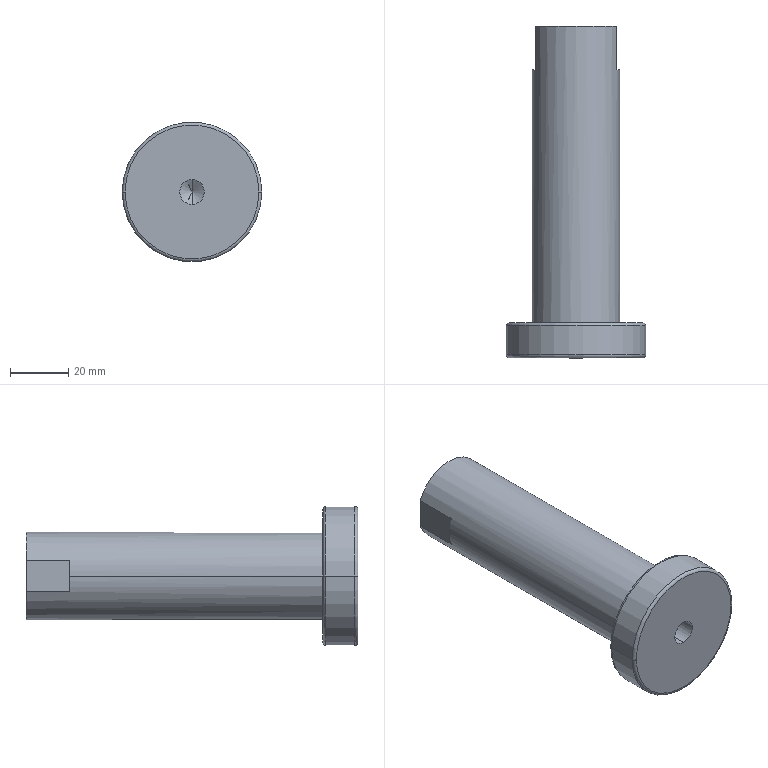Part | SolidWorks | features HoleWzd 2, Fillet 1, ICE 1, Revolution 1 | 1 solid | 23 faces | box 48 x 114 x 48 mm | volume 74222 mm3 | cylinder 8 | plane 7 | cone 4 | torus 4 | commonest cylinder face diameters 8.5 x2 24.5 x2 30 x2 48 x2
STEP:
#1=CARTESIAN_POINT('',(0.,-1.947,4.25));
#2=VERTEX_POINT('',#1);
#3=CARTESIAN_POINT('',(0.,-1.947,-4.25));
#4=VERTEX_POINT('',#3);
#5=CARTESIAN_POINT('',(0.,-1.947,0.));
#6=DIRECTION('',(0.,-1.,0.));
#7=DIRECTION('',(0.,0.,-1.));
#8=AXIS2_PLACEMENT_3D('',#5,#6,#7);
#9=CIRCLE('',#8,4.25);
#10=EDGE_CURVE('',#2,#4,#9,.T.);
#11=ORIENTED_EDGE('',*,*,#10,.F.);
#12=CARTESIAN_POINT('',(0.,-21.947,4.25));
#13=VERTEX_POINT('',#12);
#14=CARTESIAN_POINT('',(0.,-21.947,4.25));
#15=DIRECTION('',(0.,-1.,0.));
#16=VECTOR('',#15,1000.);
#17=LINE('',#14,#16);
#18=EDGE_CURVE('',#2,#13,#17,.T.);
#19=ORIENTED_EDGE('',*,*,#18,.T.);
#20=CARTESIAN_POINT('',(0.,-21.947,-4.25));
#21=VERTEX_POINT('',#20);
#22=CARTESIAN_POINT('',(0.,-21.947,0.));
#23=DIRECTION('',(0.,-1.,0.));
#24=DIRECTION('',(0.,0.,-1.));
#25=AXIS2_PLACEMENT_3D('',#22,#23,#24);
#26=CIRCLE('',#25,4.25);
#27=EDGE_CURVE('',#13,#21,#26,.T.);
#28=ORIENTED_EDGE('',*,*,#27,.T.);
#29=CARTESIAN_POINT('',(0.,-21.947,-4.25));
#30=DIRECTION('',(0.,-1.,0.));
#31=VECTOR('',#30,1000.);
#32=LINE('',#29,#31);
#33=EDGE_CURVE('',#4,#21,#32,.T.);
#34=ORIENTED_EDGE('',*,*,#33,.F.);
#35=EDGE_LOOP('',(#11,#19,#28,#34));
#36=FACE_OUTER_BOUND('',#35,.T.);
#37=CARTESIAN_POINT('',(0.,-21.947,0.));
#38=DIRECTION('',(0.,-1.,0.));
#39=DIRECTION('',(0.,0.,-1.));
#40=AXIS2_PLACEMENT_3D('',#37,#38,#39);
#41=CYLINDRICAL_SURFACE('',#40,4.25);
#42=ADVANCED_FACE('',(#36),#41,.F.);
#43=CARTESIAN_POINT('',(0.,0.6063,0.));
#44=VERTEX_POINT('',#43);
#45=CARTESIAN_POINT('',(0.,-1.947,-4.25));
#46=DIRECTION('',(0.,-0.515,-0.8572));
#47=VECTOR('',#46,1000.);
#48=LINE('',#45,#47);
#49=EDGE_CURVE('',#44,#4,#48,.T.);
#50=ORIENTED_EDGE('',*,*,#49,.F.);
#51=CARTESIAN_POINT('',(0.,-1.947,4.25));
#52=DIRECTION('',(0.,-0.515,0.8572));
#53=VECTOR('',#52,1000.);
#54=LINE('',#51,#53);
#55=EDGE_CURVE('',#44,#2,#54,.T.);
#56=ORIENTED_EDGE('',*,*,#55,.T.);
#57=ORIENTED_EDGE('',*,*,#10,.T.);
#58=EDGE_LOOP('',(#50,#56,#57));
#59=FACE_OUTER_BOUND('',#58,.T.);
#60=CARTESIAN_POINT('',(0.,-1.947,0.));
#61=DIRECTION('',(0.,-1.,0.));
#62=DIRECTION('',(0.,0.,-1.));
#63=AXIS2_PLACEMENT_3D('',#60,#61,#62);
#64=CONICAL_SURFACE('',#63,4.25,1.03);
#65=ADVANCED_FACE('',(#59),#64,.F.);
#66=CARTESIAN_POINT('',(0.,56.053,-12.25));
#67=VERTEX_POINT('',#66);
#68=CARTESIAN_POINT('',(0.,56.053,12.25));
#69=VERTEX_POINT('',#68);
#70=CARTESIAN_POINT('',(0.,56.053,0.));
#71=DIRECTION('',(0.,1.,0.));
#72=DIRECTION('',(0.,0.,1.));
#73=AXIS2_PLACEMENT_3D('',#70,#71,#72);
#74=CIRCLE('',#73,12.25);
#75=EDGE_CURVE('',#67,#69,#74,.T.);
#76=ORIENTED_EDGE('',*,*,#75,.F.);
#77=CARTESIAN_POINT('',(0.,92.053,-12.25));
#78=VERTEX_POINT('',#77);
#79=CARTESIAN_POINT('',(0.,92.053,-12.25));
#80=DIRECTION('',(0.,1.,0.));
#81=VECTOR('',#80,1000.);
#82=LINE('',#79,#81);
#83=EDGE_CURVE('',#67,#78,#82,.T.);
#84=ORIENTED_EDGE('',*,*,#83,.T.);
#85=CARTESIAN_POINT('',(0.,92.053,12.25));
#86=VERTEX_POINT('',#85);
#87=CARTESIAN_POINT('',(0.,92.053,0.));
#88=DIRECTION('',(0.,1.,0.));
#89=DIRECTION('',(0.,0.,1.));
#90=AXIS2_PLACEMENT_3D('',#87,#88,#89);
#91=CIRCLE('',#90,12.25);
#92=EDGE_CURVE('',#78,#86,#91,.T.);
#93=ORIENTED_EDGE('',*,*,#92,.T.);
#94=CARTESIAN_POINT('',(0.,92.053,12.25));
#95=DIRECTION('',(0.,1.,0.));
#96=VECTOR('',#95,1000.);
#97=LINE('',#94,#96);
#98=EDGE_CURVE('',#69,#86,#97,.T.);
#99=ORIENTED_EDGE('',*,*,#98,.F.);
#100=EDGE_LOOP('',(#76,#84,#93,#99));
#101=FACE_OUTER_BOUND('',#100,.T.);
#102=CARTESIAN_POINT('',(0.,92.053,0.));
#103=DIRECTION('',(0.,1.,0.));
#104=DIRECTION('',(0.,0.,1.));
#105=AXIS2_PLACEMENT_3D('',#102,#103,#104);
#106=CYLINDRICAL_SURFACE('',#105,12.25);
#107=ADVANCED_FACE('',(#101),#106,.F.);
#108=CARTESIAN_POINT('',(0.,48.692,0.));
#109=VERTEX_POINT('',#108);
#110=CARTESIAN_POINT('',(0.,56.053,12.25));
#111=DIRECTION('',(0.,0.515,0.8572));
#112=VECTOR('',#111,1000.);
#113=LINE('',#110,#112);
#114=EDGE_CURVE('',#109,#69,#113,.T.);
#115=ORIENTED_EDGE('',*,*,#114,.F.);
#116=CARTESIAN_POINT('',(0.,56.053,-12.25));
#117=DIRECTION('',(0.,0.515,-0.8572));
#118=VECTOR('',#117,1000.);
#119=LINE('',#116,#118);
#120=EDGE_CURVE('',#109,#67,#119,.T.);
#121=ORIENTED_EDGE('',*,*,#120,.T.);
#122=ORIENTED_EDGE('',*,*,#75,.T.);
#123=EDGE_LOOP('',(#115,#121,#122));
#124=FACE_OUTER_BOUND('',#123,.T.);
#125=CARTESIAN_POINT('',(0.,56.053,0.));
#126=DIRECTION('',(0.,1.,0.));
#127=DIRECTION('',(0.,0.,1.));
#128=AXIS2_PLACEMENT_3D('',#125,#126,#127);
#129=CONICAL_SURFACE('',#128,12.25,1.03);
#130=ADVANCED_FACE('',(#124),#129,.F.);
#131=CARTESIAN_POINT('',(24.,-10.947,0.));
#132=VERTEX_POINT('',#131);
#133=CARTESIAN_POINT('',(-24.,-10.947,0.));
#134=VERTEX_POINT('',#133);
#135=CARTESIAN_POINT('',(0.,-10.947,0.));
#136=DIRECTION('',(0.,-1.,0.));
#137=DIRECTION('',(-1.,0.,0.));
#138=AXIS2_PLACEMENT_3D('',#135,#136,#137);
#139=CIRCLE('',#138,24.);
#140=EDGE_CURVE('',#132,#134,#139,.T.);
#141=ORIENTED_EDGE('',*,*,#140,.F.);
#142=CARTESIAN_POINT('',(23.,-9.947,0.));
#143=VERTEX_POINT('',#142);
#144=CARTESIAN_POINT('',(23.,-10.947,0.));
#145=DIRECTION('',(0.,0.,1.));
#146=DIRECTION('',(1.,0.,0.));
#147=AXIS2_PLACEMENT_3D('',#144,#145,#146);
#148=CIRCLE('',#147,1.);
#149=EDGE_CURVE('',#132,#143,#148,.T.);
#150=ORIENTED_EDGE('',*,*,#149,.T.);
#151=CARTESIAN_POINT('',(-23.,-9.947,0.));
#152=VERTEX_POINT('',#151);
#153=CARTESIAN_POINT('',(0.,-9.947,0.));
#154=DIRECTION('',(0.,1.,0.));
#155=DIRECTION('',(-1.,0.,0.));
#156=AXIS2_PLACEMENT_3D('',#153,#154,#155);
#157=CIRCLE('',#156,23.);
#158=EDGE_CURVE('',#152,#143,#157,.T.);
#159=ORIENTED_EDGE('',*,*,#158,.F.);
#160=CARTESIAN_POINT('',(-23.,-10.947,0.));
#161=DIRECTION('',(0.,0.,-1.));
#162=DIRECTION('',(-1.,0.,0.));
#163=AXIS2_PLACEMENT_3D('',#160,#161,#162);
#164=CIRCLE('',#163,1.);
#165=EDGE_CURVE('',#134,#152,#164,.T.);
#166=ORIENTED_EDGE('',*,*,#165,.F.);
#167=EDGE_LOOP('',(#141,#150,#159,#166));
#168=FACE_OUTER_BOUND('',#167,.T.);
#169=CARTESIAN_POINT('',(0.,-10.947,0.));
#170=DIRECTION('',(0.,1.,0.));
#171=DIRECTION('',(-1.,0.,0.));
#172=AXIS2_PLACEMENT_3D('',#169,#170,#171);
#173=TOROIDAL_SURFACE('',#172,23.,1.);
#174=ADVANCED_FACE('',(#168),#173,.T.);
#175=CARTESIAN_POINT('',(-24.,-20.947,0.));
#176=VERTEX_POINT('',#175);
#177=CARTESIAN_POINT('',(24.,-20.947,0.));
#178=VERTEX_POINT('',#177);
#179=CARTESIAN_POINT('',(0.,-20.947,0.));
#180=DIRECTION('',(0.,1.,0.));
#181=DIRECTION('',(1.,0.,0.));
#182=AXIS2_PLACEMENT_3D('',#179,#180,#181);
#183=CIRCLE('',#182,24.);
#184=EDGE_CURVE('',#176,#178,#183,.T.);
#185=ORIENTED_EDGE('',*,*,#184,.F.);
#186=CARTESIAN_POINT('',(-23.,-21.947,0.));
#187=VERTEX_POINT('',#186);
#188=CARTESIAN_POINT('',(-23.,-20.947,0.));
#189=DIRECTION('',(0.,0.,1.));
#190=DIRECTION('',(1.,0.,0.));
#191=AXIS2_PLACEMENT_3D('',#188,#189,#190);
#192=CIRCLE('',#191,1.);
#193=EDGE_CURVE('',#176,#187,#192,.T.);
#194=ORIENTED_EDGE('',*,*,#193,.T.);
#195=CARTESIAN_POINT('',(23.,-21.947,0.));
#196=VERTEX_POINT('',#195);
#197=CARTESIAN_POINT('',(0.,-21.947,0.));
#198=DIRECTION('',(0.,-1.,0.));
#199=DIRECTION('',(1.,0.,0.));
#200=AXIS2_PLACEMENT_3D('',#197,#198,#199);
#201=CIRCLE('',#200,23.);
#202=EDGE_CURVE('',#196,#187,#201,.T.);
#203=ORIENTED_EDGE('',*,*,#202,.F.);
#204=CARTESIAN_POINT('',(23.,-20.947,0.));
#205=DIRECTION('',(0.,0.,-1.));
#206=DIRECTION('',(-1.,0.,0.));
#207=AXIS2_PLACEMENT_3D('',#204,#205,#206);
#208=CIRCLE('',#207,1.);
#209=EDGE_CURVE('',#178,#196,#208,.T.);
#210=ORIENTED_EDGE('',*,*,#209,.F.);
#211=EDGE_LOOP('',(#185,#194,#203,#210));
#212=FACE_OUTER_BOUND('',#211,.T.);
#213=CARTESIAN_POINT('',(0.,-20.947,0.));
#214=DIRECTION('',(0.,-1.,0.));
#215=DIRECTION('',(1.,0.,0.));
#216=AXIS2_PLACEMENT_3D('',#213,#214,#215);
#217=TOROIDAL_SURFACE('',#216,23.,1.);
#218=ADVANCED_FACE('',(#212),#217,.T.);
#219=CARTESIAN_POINT('',(-15.,-9.947,0.));
#220=VERTEX_POINT('',#219);
#221=CARTESIAN_POINT('',(15.,-9.947,0.));
#222=VERTEX_POINT('',#221);
#223=CARTESIAN_POINT('',(0.,-9.947,0.));
#224=DIRECTION('',(0.,1.,0.));
#225=DIRECTION('',(-1.,0.,0.));
#226=AXIS2_PLACEMENT_3D('',#223,#224,#225);
#227=CIRCLE('',#226,15.);
#228=EDGE_CURVE('',#220,#222,#227,.T.);
#229=ORIENTED_EDGE('',*,*,#228,.T.);
#230=CARTESIAN_POINT('',(15.,77.053,0.));
#231=VERTEX_POINT('',#230);
#232=CARTESIAN_POINT('',(15.,92.053,0.));
#233=DIRECTION('',(0.,1.,0.));
#234=VECTOR('',#233,1000.);
#235=LINE('',#232,#234);
#236=EDGE_CURVE('',#222,#231,#235,.T.);
#237=ORIENTED_EDGE('',*,*,#236,.T.);
#238=CARTESIAN_POINT('',(14.,77.053,5.385));
#239=VERTEX_POINT('',#238);
#240=CARTESIAN_POINT('',(0.,77.053,0.));
#241=DIRECTION('',(0.,1.,0.));
#242=DIRECTION('',(0.,0.,-1.));
#243=AXIS2_PLACEMENT_3D('',#240,#241,#242);
#244=CIRCLE('',#243,15.);
#245=EDGE_CURVE('',#239,#231,#244,.T.);
#246=ORIENTED_EDGE('',*,*,#245,.F.);
#247=CARTESIAN_POINT('',(14.,92.053,5.385));
#248=VERTEX_POINT('',#247);
#249=CARTESIAN_POINT('',(14.,92.053,5.385));
#250=DIRECTION('',(0.,-1.,0.));
#251=VECTOR('',#250,1000.);
#252=LINE('',#249,#251);
#253=EDGE_CURVE('',#248,#239,#252,.T.);
#254=ORIENTED_EDGE('',*,*,#253,.F.);
#255=CARTESIAN_POINT('',(-14.,92.053,5.385));
#256=VERTEX_POINT('',#255);
#257=CARTESIAN_POINT('',(0.,92.053,0.));
#258=DIRECTION('',(0.,1.,0.));
#259=DIRECTION('',(-1.,0.,0.));
#260=AXIS2_PLACEMENT_3D('',#257,#258,#259);
#261=CIRCLE('',#260,15.);
#262=EDGE_CURVE('',#256,#248,#261,.T.);
#263=ORIENTED_EDGE('',*,*,#262,.F.);
#264=CARTESIAN_POINT('',(-14.,77.053,5.385));
#265=VERTEX_POINT('',#264);
#266=CARTESIAN_POINT('',(-14.,92.053,5.385));
#267=DIRECTION('',(0.,1.,0.));
#268=VECTOR('',#267,1000.);
#269=LINE('',#266,#268);
#270=EDGE_CURVE('',#265,#256,#269,.T.);
#271=ORIENTED_EDGE('',*,*,#270,.F.);
#272=CARTESIAN_POINT('',(-15.,77.053,0.));
#273=VERTEX_POINT('',#272);
#274=CARTESIAN_POINT('',(0.,77.053,0.));
#275=DIRECTION('',(0.,1.,0.));
#276=DIRECTION('',(0.,0.,-1.));
#277=AXIS2_PLACEMENT_3D('',#274,#275,#276);
#278=CIRCLE('',#277,15.);
#279=EDGE_CURVE('',#273,#265,#278,.T.);
#280=ORIENTED_EDGE('',*,*,#279,.F.);
#281=CARTESIAN_POINT('',(-15.,92.053,0.));
#282=DIRECTION('',(0.,1.,0.));
#283=VECTOR('',#282,1000.);
#284=LINE('',#281,#283);
#285=EDGE_CURVE('',#220,#273,#284,.T.);
#286=ORIENTED_EDGE('',*,*,#285,.F.);
#287=EDGE_LOOP('',(#229,#237,#246,#254,#263,#271,#280,#286));
#288=FACE_OUTER_BOUND('',#287,.T.);
#289=CARTESIAN_POINT('',(0.,92.053,0.));
#290=DIRECTION('',(0.,1.,0.));
#291=DIRECTION('',(-1.,0.,0.));
#292=AXIS2_PLACEMENT_3D('',#289,#290,#291);
#293=CYLINDRICAL_SURFACE('',#292,15.);
#294=ADVANCED_FACE('',(#288),#293,.T.);
#295=ORIENTED_EDGE('',*,*,#184,.T.);
#296=CARTESIAN_POINT('',(24.,92.053,0.));
#297=DIRECTION('',(0.,1.,0.));
#298=VECTOR('',#297,1000.);
#299=LINE('',#296,#298);
#300=EDGE_CURVE('',#178,#132,#299,.T.);
#301=ORIENTED_EDGE('',*,*,#300,.T.);
#302=ORIENTED_EDGE('',*,*,#140,.T.);
#303=CARTESIAN_POINT('',(-24.,92.053,0.));
#304=DIRECTION('',(0.,1.,0.));
#305=VECTOR('',#304,1000.);
#306=LINE('',#303,#305);
#307=EDGE_CURVE('',#176,#134,#306,.T.);
#308=ORIENTED_EDGE('',*,*,#307,.F.);
#309=EDGE_LOOP('',(#295,#301,#302,#308));
#310=FACE_OUTER_BOUND('',#309,.T.);
#311=CARTESIAN_POINT('',(0.,92.053,0.));
#312=DIRECTION('',(0.,1.,0.));
#313=DIRECTION('',(-1.,0.,0.));
#314=AXIS2_PLACEMENT_3D('',#311,#312,#313);
#315=CYLINDRICAL_SURFACE('',#314,24.);
#316=ADVANCED_FACE('',(#310),#315,.T.);
#317=CARTESIAN_POINT('',(0.,92.053,0.));
#318=DIRECTION('',(0.,1.,0.));
#319=DIRECTION('',(0.,0.,1.));
#320=AXIS2_PLACEMENT_3D('',#317,#318,#319);
#321=CIRCLE('',#320,12.25);
#322=EDGE_CURVE('',#86,#78,#321,.T.);
#323=ORIENTED_EDGE('',*,*,#322,.F.);
#324=ORIENTED_EDGE('',*,*,#92,.F.);
#325=EDGE_LOOP('',(#323,#324));
#326=FACE_BOUND('',#325,.T.);
#327=CARTESIAN_POINT('',(-14.,92.053,-5.385));
#328=VERTEX_POINT('',#327);
#329=CARTESIAN_POINT('',(-14.,92.053,-24.));
#330=DIRECTION('',(0.,0.,1.));
#331=VECTOR('',#330,1000.);
#332=LINE('',#329,#331);
#333=EDGE_CURVE('',#328,#256,#332,.T.);
#334=ORIENTED_EDGE('',*,*,#333,.T.);
#335=ORIENTED_EDGE('',*,*,#262,.T.);
#336=CARTESIAN_POINT('',(14.,92.053,-5.385));
#337=VERTEX_POINT('',#336);
#338=CARTESIAN_POINT('',(14.,92.053,-24.));
#339=DIRECTION('',(0.,0.,1.));
#340=VECTOR('',#339,1000.);
#341=LINE('',#338,#340);
#342=EDGE_CURVE('',#337,#248,#341,.T.);
#343=ORIENTED_EDGE('',*,*,#342,.F.);
#344=CARTESIAN_POINT('',(0.,92.053,0.));
#345=DIRECTION('',(0.,1.,0.));
#346=DIRECTION('',(-1.,0.,0.));
#347=AXIS2_PLACEMENT_3D('',#344,#345,#346);
#348=CIRCLE('',#347,15.);
#349=EDGE_CURVE('',#337,#328,#348,.T.);
#350=ORIENTED_EDGE('',*,*,#349,.T.);
#351=EDGE_LOOP('',(#334,#335,#343,#350));
#352=FACE_OUTER_BOUND('',#351,.T.);
#353=CARTESIAN_POINT('',(-15.,92.053,0.));
#354=DIRECTION('',(0.,1.,0.));
#355=DIRECTION('',(-1.,0.,0.));
#356=AXIS2_PLACEMENT_3D('',#353,#354,#355);
#357=PLANE('',#356);
#358=ADVANCED_FACE('',(#326,#352),#357,.T.);
#359=CARTESIAN_POINT('',(0.,-21.947,0.));
#360=DIRECTION('',(0.,-1.,0.));
#361=DIRECTION('',(0.,0.,-1.));
#362=AXIS2_PLACEMENT_3D('',#359,#360,#361);
#363=CIRCLE('',#362,4.25);
#364=EDGE_CURVE('',#21,#13,#363,.T.);
#365=ORIENTED_EDGE('',*,*,#364,.F.);
#366=ORIENTED_EDGE('',*,*,#27,.F.);
#367=EDGE_LOOP('',(#365,#366));
#368=FACE_BOUND('',#367,.T.);
#369=ORIENTED_EDGE('',*,*,#202,.T.);
#370=CARTESIAN_POINT('',(0.,-21.947,0.));
#371=DIRECTION('',(0.,-1.,0.));
#372=DIRECTION('',(1.,0.,0.));
#373=AXIS2_PLACEMENT_3D('',#370,#371,#372);
#374=CIRCLE('',#373,23.);
#375=EDGE_CURVE('',#187,#196,#374,.T.);
#376=ORIENTED_EDGE('',*,*,#375,.T.);
#377=EDGE_LOOP('',(#369,#376));
#378=FACE_OUTER_BOUND('',#377,.T.);
#379=CARTESIAN_POINT('',(0.,-21.947,0.));
#380=DIRECTION('',(0.,-1.,0.));
#381=DIRECTION('',(1.,0.,0.));
#382=AXIS2_PLACEMENT_3D('',#379,#380,#381);
#383=PLANE('',#382);
#384=ADVANCED_FACE('',(#368,#378),#383,.T.);
#385=ORIENTED_EDGE('',*,*,#300,.F.);
#386=CARTESIAN_POINT('',(0.,-20.947,0.));
#387=DIRECTION('',(0.,1.,0.));
#388=DIRECTION('',(1.,0.,0.));
#389=AXIS2_PLACEMENT_3D('',#386,#387,#388);
#390=CIRCLE('',#389,24.);
#391=EDGE_CURVE('',#178,#176,#390,.T.);
#392=ORIENTED_EDGE('',*,*,#391,.T.);
#393=ORIENTED_EDGE('',*,*,#307,.T.);
#394=CARTESIAN_POINT('',(0.,-10.947,0.));
#395=DIRECTION('',(0.,-1.,0.));
#396=DIRECTION('',(-1.,0.,0.));
#397=AXIS2_PLACEMENT_3D('',#394,#395,#396);
#398=CIRCLE('',#397,24.);
#399=EDGE_CURVE('',#134,#132,#398,.T.);
#400=ORIENTED_EDGE('',*,*,#399,.T.);
#401=EDGE_LOOP('',(#385,#392,#393,#400));
#402=FACE_OUTER_BOUND('',#401,.T.);
#403=CARTESIAN_POINT('',(0.,92.053,0.));
#404=DIRECTION('',(0.,1.,0.));
#405=DIRECTION('',(-1.,0.,0.));
#406=AXIS2_PLACEMENT_3D('',#403,#404,#405);
#407=CYLINDRICAL_SURFACE('',#406,24.);
#408=ADVANCED_FACE('',(#402),#407,.T.);
#409=ORIENTED_EDGE('',*,*,#158,.T.);
#410=CARTESIAN_POINT('',(0.,-9.947,0.));
#411=DIRECTION('',(0.,1.,0.));
#412=DIRECTION('',(-1.,0.,0.));
#413=AXIS2_PLACEMENT_3D('',#410,#411,#412);
#414=CIRCLE('',#413,23.);
#415=EDGE_CURVE('',#143,#152,#414,.T.);
#416=ORIENTED_EDGE('',*,*,#415,.T.);
#417=EDGE_LOOP('',(#409,#416));
#418=FACE_OUTER_BOUND('',#417,.T.);
#419=ORIENTED_EDGE('',*,*,#228,.F.);
#420=CARTESIAN_POINT('',(0.,-9.947,0.));
#421=DIRECTION('',(0.,1.,0.));
#422=DIRECTION('',(-1.,0.,0.));
#423=AXIS2_PLACEMENT_3D('',#420,#421,#422);
#424=CIRCLE('',#423,15.);
#425=EDGE_CURVE('',#222,#220,#424,.T.);
#426=ORIENTED_EDGE('',*,*,#425,.F.);
#427=EDGE_LOOP('',(#419,#426));
#428=FACE_BOUND('',#427,.T.);
#429=CARTESIAN_POINT('',(-24.,-9.947,0.));
#430=DIRECTION('',(0.,1.,0.));
#431=DIRECTION('',(-1.,0.,0.));
#432=AXIS2_PLACEMENT_3D('',#429,#430,#431);
#433=PLANE('',#432);
#434=ADVANCED_FACE('',(#418,#428),#433,.T.);
#435=ORIENTED_EDGE('',*,*,#236,.F.);
#436=ORIENTED_EDGE('',*,*,#425,.T.);
#437=ORIENTED_EDGE('',*,*,#285,.T.);
#438=CARTESIAN_POINT('',(-14.,77.053,-5.385));
#439=VERTEX_POINT('',#438);
#440=CARTESIAN_POINT('',(0.,77.053,0.));
#441=DIRECTION('',(0.,1.,0.));
#442=DIRECTION('',(0.,0.,-1.));
#443=AXIS2_PLACEMENT_3D('',#440,#441,#442);
#444=CIRCLE('',#443,15.);
#445=EDGE_CURVE('',#439,#273,#444,.T.);
#446=ORIENTED_EDGE('',*,*,#445,.F.);
#447=CARTESIAN_POINT('',(-14.,92.053,-5.385));
#448=DIRECTION('',(0.,-1.,0.));
#449=VECTOR('',#448,1000.);
#450=LINE('',#447,#449);
#451=EDGE_CURVE('',#328,#439,#450,.T.);
#452=ORIENTED_EDGE('',*,*,#451,.F.);
#453=ORIENTED_EDGE('',*,*,#349,.F.);
#454=CARTESIAN_POINT('',(14.,77.053,-5.385));
#455=VERTEX_POINT('',#454);
#456=CARTESIAN_POINT('',(14.,92.053,-5.385));
#457=DIRECTION('',(0.,1.,0.));
#458=VECTOR('',#457,1000.);
#459=LINE('',#456,#458);
#460=EDGE_CURVE('',#455,#337,#459,.T.);
#461=ORIENTED_EDGE('',*,*,#460,.F.);
#462=CARTESIAN_POINT('',(0.,77.053,0.));
#463=DIRECTION('',(0.,1.,0.));
#464=DIRECTION('',(0.,0.,-1.));
#465=AXIS2_PLACEMENT_3D('',#462,#463,#464);
#466=CIRCLE('',#465,15.);
#467=EDGE_CURVE('',#231,#455,#466,.T.);
#468=ORIENTED_EDGE('',*,*,#467,.F.);
#469=EDGE_LOOP('',(#435,#436,#437,#446,#452,#453,#461,#468));
#470=FACE_OUTER_BOUND('',#469,.T.);
#471=CARTESIAN_POINT('',(0.,92.053,0.));
#472=DIRECTION('',(0.,1.,0.));
#473=DIRECTION('',(-1.,0.,0.));
#474=AXIS2_PLACEMENT_3D('',#471,#472,#473);
#475=CYLINDRICAL_SURFACE('',#474,15.);
#476=ADVANCED_FACE('',(#470),#475,.T.);
#477=CARTESIAN_POINT('',(14.,77.053,-24.));
#478=DIRECTION('',(0.,0.,1.));
#479=VECTOR('',#478,1000.);
#480=LINE('',#477,#479);
#481=EDGE_CURVE('',#455,#239,#480,.T.);
#482=ORIENTED_EDGE('',*,*,#481,.T.);
#483=ORIENTED_EDGE('',*,*,#245,.T.);
#484=ORIENTED_EDGE('',*,*,#467,.T.);
#485=EDGE_LOOP('',(#482,#483,#484));
#486=FACE_OUTER_BOUND('',#485,.T.);
#487=CARTESIAN_POINT('',(15.,77.053,-24.));
#488=DIRECTION('',(0.,-1.,0.));
#489=DIRECTION('',(0.,0.,-1.));
#490=AXIS2_PLACEMENT_3D('',#487,#488,#489);
#491=PLANE('',#490);
#492=ADVANCED_FACE('',(#486),#491,.F.);
#493=ORIENTED_EDGE('',*,*,#253,.T.);
#494=ORIENTED_EDGE('',*,*,#481,.F.);
#495=ORIENTED_EDGE('',*,*,#460,.T.);
#496=ORIENTED_EDGE('',*,*,#342,.T.);
#497=EDGE_LOOP('',(#493,#494,#495,#496));
#498=FACE_OUTER_BOUND('',#497,.T.);
#499=CARTESIAN_POINT('',(14.,92.053,-24.));
#500=DIRECTION('',(-1.,0.,0.));
#501=DIRECTION('',(0.,-1.,0.));
#502=AXIS2_PLACEMENT_3D('',#499,#500,#501);
#503=PLANE('',#502);
#504=ADVANCED_FACE('',(#498),#503,.F.);
#505=ORIENTED_EDGE('',*,*,#451,.T.);
#506=CARTESIAN_POINT('',(-14.,77.053,-24.));
#507=DIRECTION('',(0.,0.,1.));
#508=VECTOR('',#507,1000.);
#509=LINE('',#506,#508);
#510=EDGE_CURVE('',#439,#265,#509,.T.);
#511=ORIENTED_EDGE('',*,*,#510,.T.);
#512=ORIENTED_EDGE('',*,*,#270,.T.);
#513=ORIENTED_EDGE('',*,*,#333,.F.);
#514=EDGE_LOOP('',(#505,#511,#512,#513));
#515=FACE_OUTER_BOUND('',#514,.T.);
#516=CARTESIAN_POINT('',(-14.,92.053,-24.));
#517=DIRECTION('',(1.,0.,0.));
#518=DIRECTION('',(0.,0.,-1.));
#519=AXIS2_PLACEMENT_3D('',#516,#517,#518);
#520=PLANE('',#519);
#521=ADVANCED_FACE('',(#515),#520,.F.);
#522=ORIENTED_EDGE('',*,*,#510,.F.);
#523=ORIENTED_EDGE('',*,*,#445,.T.);
#524=ORIENTED_EDGE('',*,*,#279,.T.);
#525=EDGE_LOOP('',(#522,#523,#524));
#526=FACE_OUTER_BOUND('',#525,.T.);
#527=CARTESIAN_POINT('',(-15.,77.053,-24.));
#528=DIRECTION('',(0.,-1.,0.));
#529=DIRECTION('',(0.,0.,-1.));
#530=AXIS2_PLACEMENT_3D('',#527,#528,#529);
#531=PLANE('',#530);
#532=ADVANCED_FACE('',(#526),#531,.F.);
#533=ORIENTED_EDGE('',*,*,#193,.F.);
#534=ORIENTED_EDGE('',*,*,#391,.F.);
#535=ORIENTED_EDGE('',*,*,#209,.T.);
#536=ORIENTED_EDGE('',*,*,#375,.F.);
#537=EDGE_LOOP('',(#533,#534,#535,#536));
#538=FACE_OUTER_BOUND('',#537,.T.);
#539=CARTESIAN_POINT('',(0.,-20.947,0.));
#540=DIRECTION('',(0.,-1.,0.));
#541=DIRECTION('',(1.,0.,0.));
#542=AXIS2_PLACEMENT_3D('',#539,#540,#541);
#543=TOROIDAL_SURFACE('',#542,23.,1.);
#544=ADVANCED_FACE('',(#538),#543,.T.);
#545=ORIENTED_EDGE('',*,*,#149,.F.);
#546=ORIENTED_EDGE('',*,*,#399,.F.);
#547=ORIENTED_EDGE('',*,*,#165,.T.);
#548=ORIENTED_EDGE('',*,*,#415,.F.);
#549=EDGE_LOOP('',(#545,#546,#547,#548));
#550=FACE_OUTER_BOUND('',#549,.T.);
#551=CARTESIAN_POINT('',(0.,-10.947,0.));
#552=DIRECTION('',(0.,1.,0.));
#553=DIRECTION('',(-1.,0.,0.));
#554=AXIS2_PLACEMENT_3D('',#551,#552,#553);
#555=TOROIDAL_SURFACE('',#554,23.,1.);
#556=ADVANCED_FACE('',(#550),#555,.T.);
#557=ORIENTED_EDGE('',*,*,#120,.F.);
#558=ORIENTED_EDGE('',*,*,#114,.T.);
#559=CARTESIAN_POINT('',(0.,56.053,0.));
#560=DIRECTION('',(0.,1.,0.));
#561=DIRECTION('',(0.,0.,1.));
#562=AXIS2_PLACEMENT_3D('',#559,#560,#561);
#563=CIRCLE('',#562,12.25);
#564=EDGE_CURVE('',#69,#67,#563,.T.);
#565=ORIENTED_EDGE('',*,*,#564,.T.);
#566=EDGE_LOOP('',(#557,#558,#565));
#567=FACE_OUTER_BOUND('',#566,.T.);
#568=CARTESIAN_POINT('',(0.,56.053,0.));
#569=DIRECTION('',(0.,1.,0.));
#570=DIRECTION('',(0.,0.,1.));
#571=AXIS2_PLACEMENT_3D('',#568,#569,#570);
#572=CONICAL_SURFACE('',#571,12.25,1.03);
#573=ADVANCED_FACE('',(#567),#572,.F.);
#574=ORIENTED_EDGE('',*,*,#83,.F.);
#575=ORIENTED_EDGE('',*,*,#564,.F.);
#576=ORIENTED_EDGE('',*,*,#98,.T.);
#577=ORIENTED_EDGE('',*,*,#322,.T.);
#578=EDGE_LOOP('',(#574,#575,#576,#577));
#579=FACE_OUTER_BOUND('',#578,.T.);
#580=CARTESIAN_POINT('',(0.,92.053,0.));
#581=DIRECTION('',(0.,1.,0.));
#582=DIRECTION('',(0.,0.,1.));
#583=AXIS2_PLACEMENT_3D('',#580,#581,#582);
#584=CYLINDRICAL_SURFACE('',#583,12.25);
#585=ADVANCED_FACE('',(#579),#584,.F.);
#586=ORIENTED_EDGE('',*,*,#55,.F.);
#587=ORIENTED_EDGE('',*,*,#49,.T.);
#588=CARTESIAN_POINT('',(0.,-1.947,0.));
#589=DIRECTION('',(0.,-1.,0.));
#590=DIRECTION('',(0.,0.,-1.));
#591=AXIS2_PLACEMENT_3D('',#588,#589,#590);
#592=CIRCLE('',#591,4.25);
#593=EDGE_CURVE('',#4,#2,#592,.T.);
#594=ORIENTED_EDGE('',*,*,#593,.T.);
#595=EDGE_LOOP('',(#586,#587,#594));
#596=FACE_OUTER_BOUND('',#595,.T.);
#597=CARTESIAN_POINT('',(0.,-1.947,0.));
#598=DIRECTION('',(0.,-1.,0.));
#599=DIRECTION('',(0.,0.,-1.));
#600=AXIS2_PLACEMENT_3D('',#597,#598,#599);
#601=CONICAL_SURFACE('',#600,4.25,1.03);
#602=ADVANCED_FACE('',(#596),#601,.F.);
#603=ORIENTED_EDGE('',*,*,#18,.F.);
#604=ORIENTED_EDGE('',*,*,#593,.F.);
#605=ORIENTED_EDGE('',*,*,#33,.T.);
#606=ORIENTED_EDGE('',*,*,#364,.T.);
#607=EDGE_LOOP('',(#603,#604,#605,#606));
#608=FACE_OUTER_BOUND('',#607,.T.);
#609=CARTESIAN_POINT('',(0.,-21.947,0.));
#610=DIRECTION('',(0.,-1.,0.));
#611=DIRECTION('',(0.,0.,-1.));
#612=AXIS2_PLACEMENT_3D('',#609,#610,#611);
#613=CYLINDRICAL_SURFACE('',#612,4.25);
#614=ADVANCED_FACE('',(#608),#613,.F.);
#615=CLOSED_SHELL('',(#42,#65,#107,#130,#174,#218,#294,#316,#358,#384,#408,#434,#476,#492,#504,#521,#532,#544,#556,#573,#585,#602,#614));
#616=MANIFOLD_SOLID_BREP('',#615);
#617=CARTESIAN_POINT('',(0.,0.,0.));
#618=DIRECTION('',(0.,0.,1.));
#619=DIRECTION('',(1.,0.,0.));
#620=AXIS2_PLACEMENT_3D('',#617,#618,#619);
#621=(LENGTH_UNIT()NAMED_UNIT(*)SI_UNIT(.MILLI.,.METRE.));
#622=UNCERTAINTY_MEASURE_WITH_UNIT(LENGTH_MEASURE(0.00001),#621,'','');
#623=(NAMED_UNIT(*)PLANE_ANGLE_UNIT()SI_UNIT($,.RADIAN.));
#624=(NAMED_UNIT(*)SI_UNIT($,.STERADIAN.)SOLID_ANGLE_UNIT());
#625=(GEOMETRIC_REPRESENTATION_CONTEXT(3)GLOBAL_UNCERTAINTY_ASSIGNED_CONTEXT((#622))GLOBAL_UNIT_ASSIGNED_CONTEXT((#621,#623,#624))REPRESENTATION_CONTEXT('',''));
#626=ADVANCED_BREP_SHAPE_REPRESENTATION('',(#616,#620),#625);